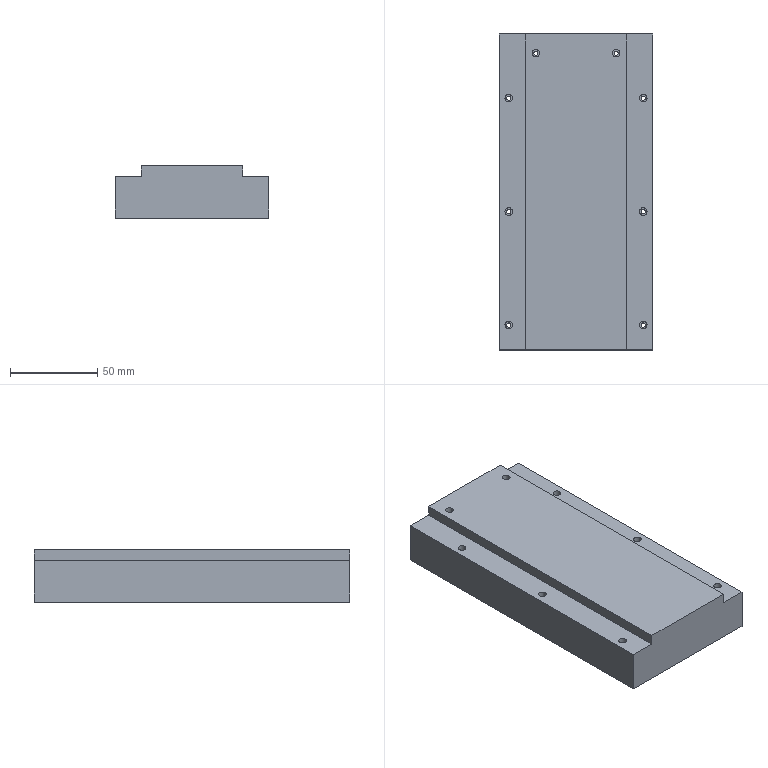NC program | NX | posted with a generic post | part box 88 x 181.05 x 30 mm
Lines 1 to 842 of 14572:
N10 G17 G21 G94 G90
(DYNAMIC_ROUGH_3_COPY_1 , TOOL : D12-36-D12-75-3T-ROUGH)
N12 T02 M6
N14 G54
N16 G17 G0 G90 X1.34 Y-53.494 B0. C0. S6500 M3
N18 G43 Z56. H2
N20 Z2.5
N22 G94 G1 X1.339 Y-53.469 Z2.344 F3000.
N24 X1.338 Y-53.444 Z2.282
N26 X1.337 Y-53.419 Z2.237
N28 Y-53.394 Z2.2
N30 X1.336 Y-53.369 Z2.169
N32 X1.335 Y-53.344 Z2.143
N34 X1.334 Y-53.319 Z2.12
N36 X1.333 Y-53.294 Z2.1
N38 X1.332 Y-53.269 Z2.082
N40 Y-53.244 Z2.067
N42 X1.331 Y-53.219 Z2.053
N44 X1.33 Y-53.194 Z2.042
N46 X1.329 Y-53.169 Z2.032
N48 X1.328 Y-53.144 Z2.023
N50 Y-53.119 Z2.016
N52 X1.327 Y-53.094 Z2.01
N54 X1.326 Y-53.069 Z2.006
N56 X1.325 Y-53.044 Z2.003
N58 X1.324 Y-53.019 Z2.001
N60 X1.323 Y-52.994 Z2.
N62 X1.261 Y-51.071
N64 G3 X0.519 Y-49.994 R1.213
N66 X-2.783 Y-49.296 R11.454
N68 X-11.156 Y-49.012 R101.327
N70 G1 X-22.823 Y-48.991
N72 X-176.793 Y-48.992
N74 G2 X-180.61 Y-47.583 R6.181
N76 X-184.883 Y-42.354 R9.042
N78 X-185.124 Y-40.599 R6.959
N80 G1 X-185.118 Y40.825
N82 G2 X-184.176 Y44.024 R7.136
N84 X-182.838 Y45.858 R8.6
N86 G1 X-181.815 Y46.797
N88 X-180.687 Y47.561
N90 G2 X-177.439 Y48.524 R8.715
N92 X-169.954 Y48.938 R68.117
N94 X-155.254 Y48.989 R897.026
N96 G1 X-2.253
N98 G2 X0.081 Y48.498 R6.42
N100 G1 X1.102 Y48.388
N102 G2 X3.166 Y47.613 R7.415
N104 X4.841 Y46.181 R7.415
N106 X5.93 Y44.264 R7.415
N108 X6.3 Y42.092 R7.42
N110 G1 Y-42.093
N112 G2 X5.929 Y-44.267 R7.418
N114 X4.84 Y-46.183 R7.415
N116 X3.163 Y-47.614 R7.415
N118 X1.1 Y-48.388 R7.415
N120 G1 X0. Y-48.497
N122 X-177.193 Y-48.496
N124 G2 X-180.208 Y-47.809 R7.763
N126 G1 X-180.666 Y-47.552
N128 G3 X-181.862 Y-47.564 R1.201
N130 G1 X-182.126 Y-47.76 Z2.014
N132 X-182.376 Y-47.974 Z2.028
N134 X-183.68 Y-49.075 Z2.1
N136 X-183.882 Y-49.246 F15000.
N138 X-184.093 Y-49.408
N140 G2 X-185.805 Y-48.929 R1.2
N142 G1 X-187.283 Y-45.973
N144 G2 X-188.766 Y-39.713 R14.05
N146 G1 X-188.886 Y36.838
N148 G2 X-188.366 Y37.828 R1.201
N150 G1 X-188.095 Y38.015
N152 X-186.147 Y39.355 Z2. F3000.
N154 X-185.829 Y39.569
N156 X-185.52 Y39.797
N158 G3 X-185.124 Y40.6 R1.203
N160 G2 X-184.505 Y43.374 R7.156
N162 X-183.796 Y44.646 R10.832
N164 X-182.838 Y45.858 R7.585
N166 G1 X-181.815 Y46.797
N168 X-180.687 Y47.561
N170 G2 X-178.403 Y48.379 R8.612
N172 G1 X-177.192 Y48.497
N174 X0.001 Y48.496
N176 X0.225 Y48.474
N178 G3 X1.49 Y49.285 R1.212
N180 G1 X2.14 Y51.167
N182 X2.148 Y51.19 Z2.001
N184 X2.156 Y51.214 Z2.003
N186 X2.164 Y51.238 Z2.006
N188 X2.172 Y51.261 Z2.01
N190 X2.18 Y51.285 Z2.016
N192 X2.189 Y51.308 Z2.023
N194 X2.197 Y51.332 Z2.032
N196 X2.205 Y51.356 Z2.042
N198 X2.213 Y51.379 Z2.053
N200 X2.221 Y51.403 Z2.067
N202 X2.229 Y51.427 Z2.082
N204 X2.238 Y51.45 Z2.1
N206 X2.246 Y51.474 Z2.12
N208 X2.254 Y51.497 Z2.143
N210 X2.262 Y51.521 Z2.169
N212 X2.27 Y51.545 Z2.2
N214 X2.278 Y51.568 Z2.237
N216 X2.287 Y51.592 Z2.282
N218 X2.295 Y51.616 Z2.344
N220 X2.303 Y51.639 Z2.5
N222 G0 Z56.
N224 X-185.914 Y47.588
N226 Z3.3
N228 G1 X-185.893 Y47.575 Z3.144
N230 X-185.872 Y47.562 Z3.082
N232 X-185.85 Y47.549 Z3.037
N234 X-185.829 Y47.536 Z3.
N236 X-185.808 Y47.522 Z2.969
N238 X-185.787 Y47.509 Z2.943
N240 X-185.765 Y47.496 Z2.92
N242 X-185.744 Y47.483 Z2.9
N244 X-185.723 Y47.47 Z2.882
N246 X-185.701 Y47.457 Z2.867
N248 X-185.68 Y47.444 Z2.853
N250 X-185.659 Y47.431 Z2.842
N252 X-185.638 Y47.418 Z2.832
N254 X-185.616 Y47.405 Z2.823
N256 X-185.595 Y47.391 Z2.816
N258 X-185.574 Y47.378 Z2.81
N260 X-185.552 Y47.365 Z2.806
N262 X-185.531 Y47.352 Z2.803
N264 X-185.51 Y47.339 Z2.801
N266 X-185.488 Y47.326 Z2.8
N268 X-183.701 Y46.226
N270 G3 X-182.368 Y46.267 R1.212
N272 G2 X-180.464 Y47.368 R7.542
N274 X-178.235 Y47.776 R7.678
N276 G1 X-11.481
N278 G3 X-4.556 Y47.608 R114.645
N280 G2 X-1.87 Y47.491 R16.77
N282 X2.298 Y44.801 R7.045
N284 X4.525 Y39.821 R12.513
N286 X5.258 Y33.271 R36.232
N288 X5.388 Y20.897 R367.986
N290 G1 X5.39 Y-38.887
N292 G2 X3.14 Y-44.025 R6.608
N294 X-1.629 Y-46.529 R11.391
N296 X-8.006 Y-47.41 R30.046
N298 G1 X-9.429 Y-47.482
N300 G2 X-11.468 Y-47.776 R7.072
N302 G1 X-178.235
N304 G2 X-180.465 Y-47.367 R7.678
N306 X-182.414 Y-46.234 R7.645
N308 G1 X-184.051 Y-45.436
N310 G3 X-185.533 Y-47.269 R1.212
N312 G1 X-185.518 Y-47.289 Z2.801
N314 X-185.502 Y-47.309 Z2.803
N316 X-185.487 Y-47.329 Z2.806
N318 X-185.472 Y-47.349 Z2.81
N320 X-185.457 Y-47.368 Z2.816
N322 X-185.441 Y-47.388 Z2.823
N324 X-185.426 Y-47.408 Z2.832
N326 X-185.411 Y-47.428 Z2.842
N328 X-185.396 Y-47.448 Z2.853
N330 X-185.381 Y-47.468 Z2.867
N332 X-185.365 Y-47.487 Z2.882
N334 X-185.35 Y-47.507 Z2.9
N336 X-185.335 Y-47.527 Z2.92
N338 X-185.32 Y-47.547 Z2.943
N340 X-185.304 Y-47.567 Z2.969
N342 X-185.289 Y-47.587 Z3.
N344 X-185.274 Y-47.606 Z3.037
N346 X-185.259 Y-47.626 Z3.082
N348 X-185.243 Y-47.646 Z3.144
N350 X-185.228 Y-47.666 Z3.3
N352 G0 Z56.
N354 X-11.915 Y51.149
N356 Z3.3
N358 G1 X-11.901 Y51.128 Z3.144
N360 X-11.887 Y51.107 Z3.082
N362 X-11.874 Y51.086 Z3.037
N364 X-11.86 Y51.066 Z3.
N366 X-11.846 Y51.045 Z2.969
N368 X-11.832 Y51.024 Z2.943
N370 X-11.818 Y51.003 Z2.92
N372 X-11.805 Y50.982 Z2.9
N374 X-11.791 Y50.961 Z2.882
N376 X-11.777 Y50.94 Z2.867
N378 X-11.763 Y50.92 Z2.853
N380 X-11.749 Y50.899 Z2.842
N382 X-11.736 Y50.878 Z2.832
N384 X-11.722 Y50.857 Z2.823
N386 X-11.708 Y50.836 Z2.816
N388 X-11.694 Y50.815 Z2.81
N390 X-11.68 Y50.795 Z2.806
N392 X-11.667 Y50.774 Z2.803
N394 X-11.653 Y50.753 Z2.801
N396 X-11.639 Y50.732 Z2.8
N398 G2 X-11.446 Y50.203 R1.234
N400 G1 X-11.276 Y48.745
N402 G3 X-10.358 Y47.707 R1.212
N404 X-7.823 Y47.105 R44.542
N406 X-4.97 Y46.757 R170.613
N408 G2 X1.178 Y42.697 R9.334
N410 X3.506 Y36.882 R15.758
N412 X4.251 Y29.654 R44.68
N414 X4.387 Y16.755 R397.795
N416 G1 X4.389 Y-36.033
N418 G2 X0.909 Y-42.957 R8.801
N420 X-4.738 Y-45.547 R14.409
N422 G3 X-6.815 Y-45.996 R53.636
N424 X-7.372 Y-46.403 R1.757
N426 G2 X-9.439 Y-47.485 R6.908
N428 G3 X-7.372 Y-46.403 R6.908
N430 G2 X-6.216 Y-45.662 R2.716
N432 G3 X-2.485 Y-44.096 R47.633
N434 X1.652 Y-40.443 R9.959
N436 X3.347 Y-35.352 R13.508
N438 X3.751 Y-28.769 R51.87
N440 X3.789 Y-18.644 R719.838
N442 G1 X3.787 Y16.156
N444 G3 X3.62 Y29.804 R338.101
N446 X2.755 Y36.865 R37.702
N448 X0.412 Y42.016 R13.406
N450 X-4.06 Y45.195 R10.315
N452 X-7.054 Y46.186 R61.029
N454 G1 X-7.308 Y46.343
N456 G2 X-7.7 Y47.194 R1.202
N458 G1 X-7.715 Y47.651
N460 X-7.789 Y50.015 Z2.9
N462 X-7.8 Y50.315 F15000.
N464 X-7.796 Y50.615
N466 G2 X-5.931 Y51.483 R1.2
N468 G1 X-5.66 Y51.302
N470 X-5.397 Y51.108
N472 G2 X-5.98 Y49.036 R1.2
N474 X-6.686 Y49.113 Z2.87 R1.32 F3000.
N476 G1 X-8.249 Y49.627 Z2.8
N478 G3 X-8.927 Y49.742 R1.544
N480 X-9.291 Y47.448 R1.2
N482 G2 X-7.37 Y46.401 R7.336
N484 G3 X-5.987 Y45.381 R6.207
N486 G2 X-2.65 Y43.055 R18.551
N488 X1.173 Y36.847 R14.372
N490 X2.451 Y29.777 R30.792
N492 X2.772 Y19.059 R150.392
N494 G1 X2.788 Y8.634
N496 X2.787 Y-21.216
N498 G2 X2.633 Y-31.264 R199.606
N500 X1.846 Y-36.29 R20.815
N502 X-2.176 Y-41.797 R11.259
N504 X-5.332 Y-43.873 R39.119
N506 G3 X-5.924 Y-44.763 R2.273
N508 G1 X-6.577 Y-45.647
N510 X-7.066 Y-46.112
N512 G3 X-5.573 Y-44.064 R5.862
N514 G2 X-4.252 Y-42.792 R9.294
N516 G3 X-1.107 Y-39.69 R19.651
N518 X1.473 Y-33.639 R14.487
N520 X2.109 Y-26.701 R41.915
N522 X2.188 Y-14.627 R570.626
N524 G1 X2.186 Y13.123
N526 G3 X2.015 Y26.546 R343.845
N528 X1.14 Y34.136 R43.737
N530 X-1.597 Y40.417 R16.378
N532 X-5.051 Y43.773 R17.766
N534 G2 X-5.771 Y44.455 R2.419
N536 G3 X-7.064 Y46.11 R5.554
N538 G2 X-5.57 Y44.052 R5.829
N540 G3 X-3.826 Y41.669 R35.059
N542 G2 X0.199 Y32.303 R22.148
N544 X1.045 Y23.578 R56.766
N546 X1.186 Y8.279 R501.856
N548 G1 X1.187 Y-15.346
N550 G2 X1.044 Y-27.419 R288.361
N552 X0.218 Y-33.577 R29.409
N554 X-3.16 Y-39.78 R15.598
N556 G3 X-4.919 Y-41.853 R39.593
N558 X-5.123 Y-42.728 R1.968
N560 G1 X-5.435 Y-43.781
N562 X-5.635 Y-44.184
N564 G3 X-5.043 Y-42.051 R5.606
N566 G2 X-4.014 Y-40.214 R8.071
N568 G3 X-1.395 Y-35.654 R25.306
N570 X0.227 Y-28.664 R24.206
N572 X0.569 Y-19.599 R102.656
N574 G1 X0.587 Y-11.274
N576 X0.585 Y9.201
N578 G3 X0.402 Y24.124 R379.325
N580 X-0.534 Y32.386 R49.502
N582 X-4.4 Y41.184 R23.99
N584 G2 X-5.053 Y42.275 R5.432
N586 G3 X-5.434 Y43.778 R7.76
N588 G1 X-5.601 Y44.114
N590 G2 X-5.046 Y42.048 R5.545
N592 G3 X-4.166 Y39.554 R14.319
N594 G2 X-0.874 Y26.642 R38.799
N596 X-0.446 Y15.553 R138.342
N598 G1 X-0.414 Y3.328
N600 X-0.415 Y-13.697
N602 G2 X-0.596 Y-25.394 R237.118
N604 X-1.633 Y-32.429 R32.419
N606 X-3.902 Y-37.734 R24.937
N608 G3 X-4.958 Y-39.817 R17.087
N610 G1 X-4.999 Y-40.062
N612 Y-41.637
N614 X-5.058 Y-42.158
N616 X-4.999 Y-41.637
N618 X-4.998 Y-39.837
N620 G2 X-4.209 Y-37.442 R10.717
N622 G3 X-1.995 Y-30.782 R34.785
N624 X-1.127 Y-22.363 R49.354
N626 X-1.014 Y-8.489 R485.88
N628 G1 X-1.016 Y7.111
N630 G3 X-1.198 Y21.884 R397.195
N632 X-2.211 Y31.27 R59.307
N634 X-4.49 Y38.639 R44.926
N636 G2 X-4.996 Y40.167 R9.609
N638 G3 X-5.05 Y42.082 R13.976
N640 G2 X-4.999 Y40.216 R12.797
N642 G3 X-4.637 Y37.174 R10.92
N644 G2 X-3.121 Y30.25 R111.025
N646 X-2.15 Y19.051 R81.729
N648 X-2.015 Y-0.073 R737.621
N650 G1 X-2.017 Y-11.698
N652 G2 X-2.229 Y-23.694 R225.827
N654 X-4.669 Y-35.583 R38.078
N656 G3 X-4.999 Y-36.694 R5.346
N658 G1 Y-39.919
N660 X-4.985 Y-36.187
N662 G2 X-4.241 Y-32.6 R30.96
N664 G3 X-2.761 Y-21.165 R55.346
N666 X-2.617 Y-8.266 R382.562
N668 G1 X-2.616 Y1.934
N670 G3 X-2.775 Y19.332 R569.007
N672 X-3.973 Y31.261 R76.778
N674 G1 X-4.999 Y36.128
N676 Y39.428
N678 G3 X-4.981 Y33.248 R319.2
N680 X-4.306 Y26.692 R271.928
N682 G2 X-3.659 Y12.086 R165.03
N684 X-3.616 Y-2.314 R932.939
N686 G1 Y-30.412
N688 G3 X-3.473 Y-30.98 R1.218
N690 X-2.455 Y-31.617 Z2.853 R1.243
N692 G1 X-1.354 Y-31.754 Z2.9
N694 X1.055 Y-32.056 F15000.
N696 G2 X0.146 Y-34.175 R-1.2
N698 G1 X-0.184 Y-33.901
N700 X-0.525 Y-33.639
N702 G3 X-2.023 Y-33.837 R1.2
N704 X-2.357 Y-34.621 Z2.863 R1.283 F3000.
N706 G1 X-2.551 Y-36.104 Z2.8
N708 X-2.589 Y-36.409
N710 X-2.642 Y-36.711
N712 G2 X-4.999 Y-36.394 R1.2
N714 X-4.641 Y-32.159 R19.712
N716 G3 X-4.252 Y-25.499 R53.938
N718 X-4.216 Y-14.25 R779.238
N720 G1 Y27.589
N722 G2 X-4.137 Y28.018 R1.28
N724 G1 X-3.239 Y30.363
N726 X-2.732 Y31.675 Z2.86
N728 G2 X-2.048 Y32.308 Z2.9 R1.2
N730 X-0.454 Y31.351 R1.2 F15000.
N732 G1 X-0.409 Y31.052
N734 X-0.379 Y30.751
N736 G2 X-2.024 Y29.632 R1.2
N738 X-2.776 Y30.824 Z2.836 R1.207 F3000.
N740 G1 X-2.721 Y31.68 Z2.8
N742 X-2.602 Y33.5
N744 G3 X-4.999 Y33.578 R-1.2
N746 G1 Y-35.122
N748 G3 X-3.956 Y-36.322 R1.212
N750 G1 X-2.043 Y-36.592
N752 X-2.019 Y-36.595 Z2.801
N754 X-1.994 Y-36.599 Z2.803
N756 X-1.969 Y-36.602 Z2.806
N758 X-1.944 Y-36.606 Z2.81
N760 X-1.92 Y-36.609 Z2.816
N762 X-1.895 Y-36.613 Z2.823
N764 X-1.87 Y-36.616 Z2.832
N766 X-1.845 Y-36.62 Z2.842
N768 X-1.82 Y-36.623 Z2.853
N770 X-1.796 Y-36.627 Z2.867
N772 X-1.771 Y-36.63 Z2.882
N774 X-1.746 Y-36.634 Z2.9
N776 X-1.721 Y-36.637 Z2.92
N778 X-1.697 Y-36.641 Z2.943
N780 X-1.672 Y-36.644 Z2.969
N782 X-1.647 Y-36.648 Z3.
N784 X-1.622 Y-36.651 Z3.037
N786 X-1.598 Y-36.655 Z3.082
N788 X-1.573 Y-36.658 Z3.144
N790 X-1.548 Y-36.662 Z3.3
N792 G0 Z56.
N794 X-29.333 Y-20.835
N796 Z4.5
N798 G1 X-29.326 Y-20.859 Z4.344
N800 X-29.318 Y-20.883 Z4.282
N802 X-29.311 Y-20.907 Z4.237
N804 X-29.303 Y-20.931 Z4.2
N806 X-29.296 Y-20.955 Z4.169
N808 X-29.289 Y-20.979 Z4.143
N810 X-29.281 Y-21.003 Z4.12
N812 X-29.274 Y-21.026 Z4.1
N814 X-29.267 Y-21.05 Z4.082
N816 X-29.259 Y-21.074 Z4.067
N818 X-29.252 Y-21.098 Z4.053
N820 X-29.245 Y-21.122 Z4.042
N822 X-29.237 Y-21.146 Z4.032
N824 X-29.23 Y-21.17 Z4.023
N826 X-29.222 Y-21.194 Z4.016
N828 X-29.215 Y-21.218 Z4.01
N830 X-29.208 Y-21.241 Z4.006
N832 X-29.2 Y-21.265 Z4.003
N834 X-29.193 Y-21.289 Z4.001
N836 X-29.186 Y-21.313 Z4.
N838 X-28.437 Y-23.741
N840 G3 X-26.621 Y-24.402 R1.212
N842 X-26.077 Y-23.645 R1.37
N844 X-25.493 Y-20.583 R12.511
N846 G1 X-25.507 Y22.575
N848 G3 X-26.205 Y24.386 R3.079
N850 X-26.719 Y24.684 R1.494
N852 X-28.34 Y23.101 R1.32
N854 G1 X-28.096 Y22.084
N856 G3 X-25.493 Y22.392 R1.32
N858 X-25.545 Y23.631 R5.91
N860 X-26.853 Y24.783 R1.384
N862 X-27.447 Y22.068 R1.436
N864 X-25.493 Y23.292 R1.36
N866 X-27.04 Y24.769 R1.32
N868 X-27.966 Y24.08 R1.201
N870 G1 X-28.252 Y23.456
N872 X-29.236 Y21.305 Z4.1
N874 G3 X-29.367 Y20.737 R1.239 F15000.
N876 G1 X-28.784 Y-17.291
N878 G3 X-28.464 Y-18.09 R1.203
N880 X-28. Y-18.421 Z4.076 R1.886 F3000.
N882 G1 X-26.456 Y-19.33 Z4.
N884 X-26.202 Y-19.478
N886 X-25.955 Y-19.637
N888 G2 X-25.493 Y-20.583 R1.201
N890 X-25.553 Y-22.677 R15.085
N892 X-26.401 Y-24.453 R2.882
N894 G1 X-26.658 Y-24.607
N896 G2 X-28.339 Y-23.139 R1.223
N898 G1 X-27.884 Y-21.651
N900 G2 X-25.493 Y-22.008 R1.223
N902 X-25.617 Y-23.49 R4.537
N904 X-26.609 Y-24.677 R1.744
N906 G1 X-26.753 Y-24.718
N908 G2 X-28.263 Y-22.999 R1.32
N910 G1 X-28.136 Y-22.62
N912 X-27.995 Y-22.246
N914 G2 X-25.493 Y-22.833 R1.32
N916 X-26.178 Y-24.55 R1.912
N918 X-26.882 Y-24.774 R1.368
N920 X-28.061 Y-22.976 R1.275
N922 G1 X-27.96 Y-22.752
N924 X-27.849 Y-22.532
N926 G2 X-25.493 Y-23.208 R1.275
N928 X-26.407 Y-24.729 R1.415
N930 X-27.04 Y-24.769 R1.46
N932 G3 X-26.596 Y-24.774 R1.283
N934 X-25.496 Y-23.545 R1.269
N936 X-26.171 Y-22.39 R1.212
N938 G1 X-28.456 Y-21.266
N940 X-28.479 Y-21.255 Z4.001
N942 X-28.501 Y-21.244 Z4.003
N944 X-28.523 Y-21.233 Z4.006
N946 X-28.546 Y-21.221 Z4.01
N948 X-28.568 Y-21.21 Z4.016
N950 X-28.591 Y-21.199 Z4.023
N952 X-28.613 Y-21.188 Z4.032
N954 X-28.636 Y-21.177 Z4.042
N956 X-28.658 Y-21.166 Z4.053
N958 X-28.68 Y-21.155 Z4.067
N960 X-28.703 Y-21.144 Z4.082
N962 X-28.725 Y-21.133 Z4.1
N964 X-28.748 Y-21.122 Z4.12
N966 X-28.77 Y-21.111 Z4.143
N968 X-28.793 Y-21.1 Z4.169
N970 X-28.815 Y-21.089 Z4.2
N972 X-28.838 Y-21.078 Z4.237
N974 X-28.86 Y-21.067 Z4.282
N976 X-28.882 Y-21.056 Z4.344
N978 X-28.905 Y-21.045 Z4.5
N980 G0 Z56.
N982 X-11.107 Y-51.291
N984 Z3.5
N986 G1 X-11.108 Y-51.266 Z3.344
N988 X-11.109 Y-51.241 Z3.282
N990 X-11.11 Y-51.216 Z3.237
N992 X-11.111 Y-51.191 Z3.2
N994 X-11.113 Y-51.166 Z3.169
N996 X-11.114 Y-51.141 Z3.143
N998 X-11.115 Y-51.116 Z3.12
N1000 X-11.116 Y-51.091 Z3.1
N1002 X-11.117 Y-51.066 Z3.082
N1004 X-11.118 Y-51.041 Z3.067
N1006 X-11.12 Y-51.016 Z3.053
N1008 X-11.121 Y-50.991 Z3.042
N1010 X-11.122 Y-50.966 Z3.032
N1012 X-11.123 Y-50.941 Z3.023
N1014 X-11.124 Y-50.916 Z3.016
N1016 X-11.126 Y-50.891 Z3.01
N1018 X-11.127 Y-50.866 Z3.006
N1020 X-11.128 Y-50.841 Z3.003
N1022 X-11.129 Y-50.816 Z3.001
N1024 X-11.13 Y-50.791 Z3.
N1026 X-11.223 Y-48.838
N1028 G3 X-11.934 Y-47.79 R1.213
N1030 X-12.556 Y-47.603 R2.105
N1032 G1 X-178.416
N1034 G2 X-180.6 Y-47.208 R7.266
N1036 X-182.507 Y-46.074 R7.263
N1038 X-183.896 Y-44.344 R7.263
N1040 X-184.682 Y-41.314 R7.193
N1042 G1 X-184.681 Y41.314
N1044 G2 X-184.3 Y43.467 R7.323
N1046 X-183.206 Y45.358 R7.32
N1048 X-181.531 Y46.762 R7.32
N1050 X-179.477 Y47.508 R7.32
N1052 G1 X-178.385 Y47.603
N1054 X-12.324
N1056 G2 X-10.133 Y47.275 R7.387
N1058 X-8.213 Y46.228 R7.336
N1060 X-6.766 Y44.588 R7.336
N1062 X-5.966 Y42.552 R7.336
N1064 X-5.876 Y39.283 R15.108
N1066 G1 X-5.922 Y37.594
N1068 G2 X-5.841 Y36.758 R13.426
N1070 G1 X-5.84 Y-36.872
N1072 X-5.945 Y-39.243
N1074 G2 X-5.966 Y-42.555 R11.029
N1076 X-6.767 Y-44.59 R7.336
N1078 X-8.215 Y-46.23 R7.336
N1080 X-10.136 Y-47.276 R7.336
N1082 X-12.311 Y-47.603 R7.333
N1084 G1 X-12.611
N1086 X-11.203 Y-47.534
N1088 G3 X-9.13 Y-46.837 R7.336
N1090 X-7.419 Y-45.473 R7.336
N1092 X-6.278 Y-43.607 R7.336
N1094 X-5.842 Y-41.462 R7.337
N1096 X-5.967 Y-38.985 R13.049
N1098 G2 X-5.84 Y-36.872 R10.37
N1100 X-5.296 Y-36.002 R1.202
N1102 G1 X-4.858 Y-35.721
N1104 X-3.044 Y-34.551 Z3.091
N1106 X-2.887 Y-34.418 Z3.1
N1108 G3 X-2.548 Y-33.58 R1.203 F15000.
N1110 G1 X-2.631 Y34.302
N1112 G3 X-2.868 Y35.017 R1.207
N1114 X-3.276 Y35.371 Z3.077 R1.414 F3000.
N1116 G1 X-4.805 Y36.358 Z3.
N1118 X-5.158 Y36.583
N1120 X-5.503 Y36.819
N1122 G2 X-5.922 Y37.594 R1.203
N1124 X-5.838 Y40.146 R9.14
N1126 X-4.934 Y41.177 R1.212
N1128 G1 X-2.899 Y41.696
N1130 X-2.875 Y41.702 Z3.001
N1132 X-2.851 Y41.709 Z3.003
N1134 X-2.826 Y41.715 Z3.006
N1136 X-2.802 Y41.721 Z3.01
N1138 X-2.778 Y41.727 Z3.016
N1140 X-2.754 Y41.733 Z3.023
N1142 X-2.73 Y41.74 Z3.032
N1144 X-2.705 Y41.746 Z3.042
N1146 X-2.681 Y41.752 Z3.053
N1148 X-2.657 Y41.758 Z3.067
N1150 X-2.633 Y41.764 Z3.082
N1152 X-2.608 Y41.77 Z3.1
N1154 X-2.584 Y41.777 Z3.12
N1156 X-2.56 Y41.783 Z3.143
N1158 X-2.536 Y41.789 Z3.169
N1160 X-2.512 Y41.795 Z3.2
N1162 X-2.487 Y41.801 Z3.237
N1164 X-2.463 Y41.808 Z3.282
N1166 X-2.439 Y41.814 Z3.344
N1168 X-2.415 Y41.82 Z3.5
N1170 G0 Z56.
N1172 X-15.485 Y-51.118
N1174 Z4.5
N1176 G1 X-15.486 Y-51.093 Z4.344
N1178 X-15.488 Y-51.068 Z4.282
N1180 X-15.489 Y-51.043 Z4.237
N1182 X-15.49 Y-51.018 Z4.2
N1184 X-15.492 Y-50.993 Z4.169
N1186 X-15.493 Y-50.968 Z4.143
N1188 X-15.495 Y-50.943 Z4.12
N1190 X-15.496 Y-50.918 Z4.1
N1192 X-15.497 Y-50.893 Z4.082
N1194 X-15.499 Y-50.868 Z4.067
N1196 X-15.5 Y-50.843 Z4.053
N1198 X-15.501 Y-50.818 Z4.042
N1200 X-15.503 Y-50.793 Z4.032
N1202 X-15.504 Y-50.768 Z4.023
N1204 X-15.506 Y-50.743 Z4.016
N1206 X-15.507 Y-50.718 Z4.01
N1208 X-15.508 Y-50.693 Z4.006
N1210 X-15.51 Y-50.668 Z4.003
N1212 X-15.511 Y-50.643 Z4.001
N1214 X-15.513 Y-50.618 Z4.
N1216 X-15.622 Y-48.647
N1218 G3 X-16.317 Y-47.618 R1.213
N1220 X-19.106 Y-46.965 R9.276
N1222 X-23.208 Y-46.703 R55.536
N1224 G1 X-77.457 Y-46.705
N1226 G3 X-79.265 Y-46.703 R10.908
N1228 G1 X-177.979 Y-46.702
N1230 G2 X-180.119 Y-46.315 R7.288
N1232 X-181.998 Y-45.22 R7.285
N1234 X-183.389 Y-43.548 R7.285
N1236 X-184.125 Y-41.501 R7.285
N1238 G1 X-184.215 Y-40.412
N1240 Y40.412
N1242 G2 X-183.846 Y42.559 R7.292
N1244 X-182.765 Y44.447 R7.285
N1246 X-181.105 Y45.851 R7.285
N1248 X-179.064 Y46.603 R7.285
N1250 G1 X-177.977 Y46.702
N1252 X-79.261 Y46.704
N1254 G3 X-77.335 Y46.703 R13.522
N1256 G1 X-16.702 Y46.702
N1258 G2 X-14.419 Y46.598 R96.553
N1260 X-10.161 Y44.071 R6.634
N1262 X-7.655 Y38.504 R13.216
N1264 X-6.968 Y32.023 R37.881
N1266 X-6.844 Y19.874 R380.762
N1268 G1 X-6.842 Y-33.226
N1270 G3 X-6.894 Y-38.571 R165.405
N1272 G2 X-8.947 Y-42.877 R6.484
N1274 X-12.007 Y-44.817 R9.165
N1276 G3 X-12.593 Y-45.329 R4.428
N1278 G2 X-14.514 Y-46.376 R7.336
N1280 X-16.689 Y-46.703 R7.333
N1282 G1 X-23.214
N1284 X-16.689
N1286 G3 X-14.514 Y-46.376 R7.36
N1288 X-12.593 Y-45.329 R7.336
N1290 G1 X-10.758 Y-43.63
N1292 G3 X-8.34 Y-39.044 R10.444
N1294 X-7.55 Y-32.883 R28.137
N1296 X-7.443 Y-19.834 R404.652
N1298 G1 X-7.445 Y19.991
N1300 G3 X-7.608 Y32.289 R283.811
N1302 X-8.415 Y38.375 R29.959
N1304 X-9.907 Y41.791 R10.146
N1306 G1 X-10.663 Y42.722
N1308 G3 X-11.796 Y44.571 R7.249
N1310 X-13.505 Y45.935 R7.336
N1312 X-15.578 Y46.633 R7.336
N1314 G1 X-16.177 Y46.67
N1316 X-15.578 Y46.633
N1318 G2 X-13.505 Y45.935 R7.336
N1320 X-11.796 Y44.571 R7.336
N1322 X-10.655 Y42.705 R7.336
N1324 X-8.647 Y30.846 R45.188
N1326 X-8.45 Y18.699 R276.781
N1328 G1 X-8.443 Y10.449
N1330 X-8.448 Y-35.751
N1332 G2 X-10.147 Y-40.16 R18.014
N1334 G3 X-10.344 Y-41.654 R10.771
N1336 G2 X-11.145 Y-43.69 R7.336
N1338 G1 X-11.797 Y-44.573
N1340 X-12.015 Y-44.779
N1342 X-11.797 Y-44.573
N1344 G3 X-10.656 Y-42.707 R7.336
N1346 X-10.218 Y-40.289 R7.174
N1348 G1 X-9.626 Y-37.72
N1350 G3 X-9.102 Y-31.374 R39.225
N1352 X-9.044 Y-18.924 R760.897
N1354 G1 X-9.049 Y34.571
N1356 G3 X-9.54 Y36.242 R53.443
N1358 G2 X-10.22 Y38.923 R37.111
N1360 G1 Y40.561
N1362 X-10.344 Y41.652
N1364 X-10.22 Y40.561
N1366 G3 X-10.122 Y34.568 R105.956
N1368 G2 X-10.044 Y18.518 R867.565
N1370 G1 X-10.049 Y-34.38
N1372 X-10.22 Y-35.365
N1374 Y-40.39
N1376 Y37.31
N1378 G2 X-8.968 Y38.521 R1.212
N1380 G1 X-7.264 Y38.465
N1382 X-7.239 Y38.464 Z4.001
N1384 X-7.214 Y38.463 Z4.003
N1386 X-7.189 Z4.006
N1388 X-7.164 Y38.462 Z4.01
N1390 X-7.139 Y38.461 Z4.016
N1392 X-7.114 Y38.46 Z4.023
N1394 X-7.089 Y38.459 Z4.032
N1396 X-7.064 Y38.458 Z4.042
N1398 X-7.039 Z4.053
N1400 X-7.014 Y38.457 Z4.067
N1402 X-6.989 Y38.456 Z4.082
N1404 X-6.964 Y38.455 Z4.1
N1406 X-6.939 Y38.454 Z4.12
N1408 X-6.914 Y38.453 Z4.143
N1410 X-6.889 Z4.169
N1412 X-6.864 Y38.452 Z4.2
N1414 X-6.839 Y38.451 Z4.237
N1416 X-6.814 Y38.45 Z4.282
N1418 X-6.789 Y38.449 Z4.344
N1420 X-6.764 Y38.448 Z4.5
N1422 G0 Z56.
N1424 X-28.849 Y-20.957
N1426 Z5.5
N1428 G1 X-28.839 Y-20.98 Z5.344
N1430 X-28.83 Y-21.004 Z5.282
N1432 X-28.821 Y-21.027 Z5.237
N1434 X-28.811 Y-21.05 Z5.2
N1436 X-28.802 Y-21.073 Z5.169
N1438 X-28.793 Y-21.096 Z5.143
N1440 X-28.783 Y-21.119 Z5.12
N1442 X-28.774 Y-21.143 Z5.1
N1444 X-28.765 Y-21.166 Z5.082
N1446 X-28.755 Y-21.189 Z5.067
N1448 X-28.746 Y-21.212 Z5.053
N1450 X-28.737 Y-21.235 Z5.042
N1452 X-28.727 Y-21.259 Z5.032
N1454 X-28.718 Y-21.282 Z5.023
N1456 X-28.709 Y-21.305 Z5.016
N1458 X-28.699 Y-21.328 Z5.01
N1460 X-28.69 Y-21.351 Z5.006
N1462 X-28.681 Y-21.375 Z5.003
N1464 X-28.671 Y-21.398 Z5.001
N1466 X-28.662 Y-21.421 Z5.
N1468 X-27.578 Y-24.109
N1470 G3 X-26.707 Y-24.841 R1.213
N1472 X-25.433 Y-24.028 R1.192
N1474 X-24.81 Y-20.999 R11.255
N1476 X-24.515 Y-12.798 R96.255
N1478 G1 X-24.493 Y-2.481
N1480 X-24.495 Y20.65
N1482 G3 X-24.818 Y23.399 R8.932
N1484 X-25.886 Y24.771 R2.27
N1486 X-26.546 Y24.871 R1.488
N1488 X-27.537 Y23.982 R1.2
N1490 G1 X-27.579 Y23.817
N1492 X-28.168 Y21.527 Z5.1
N1494 X-28.236 Y21.262 F15000.
N1496 X-28.314 Y21.
N1498 G2 X-29.207 Y20.263 R1.201
N1500 X-30.022 Y20.293 R1.368
N1502 X-30.709 Y20.982 R1.202
N1504 X-30.291 Y22.386 Z5.033 R1.205 F3000.
N1506 G1 X-29.651 Y22.847 Z5.
N1508 X-27.166 Y24.639
N1510 G2 X-26.706 Y24.841 R1.244
N1512 X-25.388 Y24.526 R1.284
N1514 X-24.398 Y22.663 R3.556
N1516 X-23.988 Y18.649 R21.637
N1518 X-23.893 Y8.727 R357.877
N1520 G1 X-23.894 Y-5.967
N1522 G2 X-24.059 Y-18.303 R275.89
N1524 X-24.636 Y-22.847 R22.716
N1526 X-25.624 Y-24.612 R3.439
N1528 X-26.54 Y-24.871 R1.315
N1530 X-27.527 Y-24.046 R1.201
N1532 X-27.515 Y-23.265 Z5.034 R1.29
N1534 G1 X-27.112 Y-21.747 Z5.1
N1536 X-27.018 Y-21.405 F15000.
N1538 X-26.941 Y-21.058
N1540 G3 X-27.917 Y-19.732 R1.2
N1542 X-28.574 Y-19.714 R1.454
N1544 X-29.443 Y-21.244 R1.2
N1546 X-29.177 Y-21.731 Z5.076 R1.909 F3000.
N1548 G1 X-28.182 Y-23.24 Z5.
N1550 X-27.467 Y-24.326
N1552 G3 X-26.707 Y-24.841 R1.203
N1554 X-25.23 Y-24.48 R1.39
N1556 X-24.005 Y-22.291 R5.101
N1558 X-23.18 Y-17.315 R22.486
N1560 X-22.906 Y-7.188 R152.907
N1562 G1 X-22.894 Y0.594
N1564 G3 X-22.966 Y16.949 R779.854
N1566 X-23.395 Y21.645 R27.246
N1568 X-24.628 Y24.348 R5.761
N1570 X-25.85 Y24.994 R1.673
N1572 X-26.524 Y24.878 R11.864
N1574 G2 X-25.638 Y25.028 R5.977
N1576 X-24.318 Y24.227 R2.234
N1578 X-23.039 Y21.538 R6.409
N1580 X-22.425 Y16.286 R27.146
N1582 X-22.293 Y4.603 R317.214
N1584 X-22.396 Y-13.017 R745.744
N1586 X-22.982 Y-20.053 R49.012
N1588 X-24.173 Y-23.594 R10.53
N1590 X-25.535 Y-24.892 R3.093
N1592 X-26.44 Y-24.895 R1.498
N1594 G3 X-25.482 Y-24.98 R2.108
N1596 X-23.852 Y-23.746 R3.124
N1598 X-22.355 Y-20.271 R9.77
N1600 X-21.516 Y-13.683 R36.298
N1602 X-21.299 Y-0.373 R280.106
N1604 X-21.403 Y14.744 R503.532
N1606 X-22.01 Y20.616 R32.955
N1608 X-23.451 Y23.995 R8.567
N1610 X-24.785 Y25.079 R3.141
N1612 X-25.342 Y25.121 R1.769
N1614 G1 X-26.003 Y24.985
N1616 X-25.046 Y25.167
N1618 G2 X-23.538 Y24.38 R2.469
N1620 X-21.972 Y21.781 R7.153
N1622 G3 X-20.444 Y20.62 R3.144
N1624 X-15.628 Y21.12 R5.349
N1626 X-12.184 Y25.382 R8.65
N1628 X-11.057 Y30.718 R18.288
N1630 X-10.859 Y38.588 R84.113
N1632 X-13.486 Y43.302 R6.792
N1634 X-18.38 Y45.462 R11.374
N1636 X-24.07 Y46.022 R31.877
N1638 X-36.97 Y46.103 R556.768
N1640 G1 X-74.788
N1642 X-84.366 Y46.102
N1644 X-175.566 Y46.101
N1646 G3 X-177.541 Y45.799 R7.154
N1648 X-179.651 Y45.416 R7.155
N1650 X-181.53 Y44.321 R7.285
N1652 X-182.922 Y42.649 R7.285
N1654 X-183.658 Y40.602 R7.285
N1656 G1 X-183.749 Y39.513
N1658 Y-39.512
N1660 G3 X-183.38 Y-41.655 R7.289
N1662 X-182.301 Y-43.544 R7.285
N1664 X-180.641 Y-44.949 R7.285
N1666 X-177.409 Y-45.841 R7.26
N1668 X-169.015 Y-46.092 R103.706
N1670 G1 X-160.915 Y-46.102
N1672 X-81.565 Y-46.101
N1674 X-71.674 Y-46.102
N1676 X-19.003 Y-46.104
N1678 G3 X-13.947 Y-43.8 R6.628
N1680 X-11.568 Y-38.979 R10.795
N1682 X-10.909 Y-32.95 R30.986